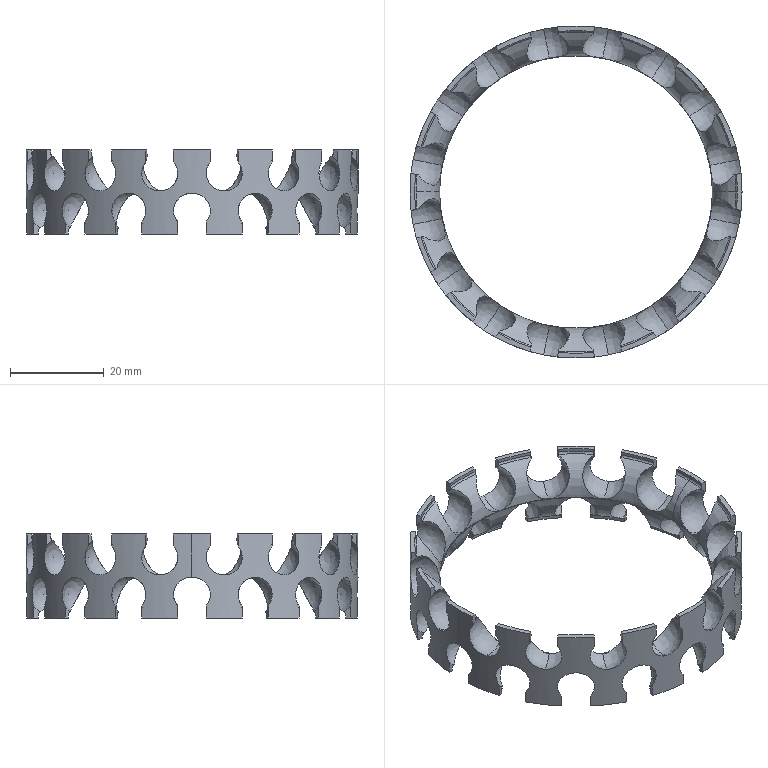Part | SolidWorks | features CirPattern 2, ICE 2, CombineBodies 1, Extrusion 1, MoveCopyBody 1, RevCut 1, Revolution 1, Stock 1 | 1 solid | 266 faces | box 71 x 71 x 18 mm | volume 5623 mm3 | plane 96 | torus 71 | sphere 64 | cylinder 35 | commonest cylinder face diameters 69 x33 71 x2